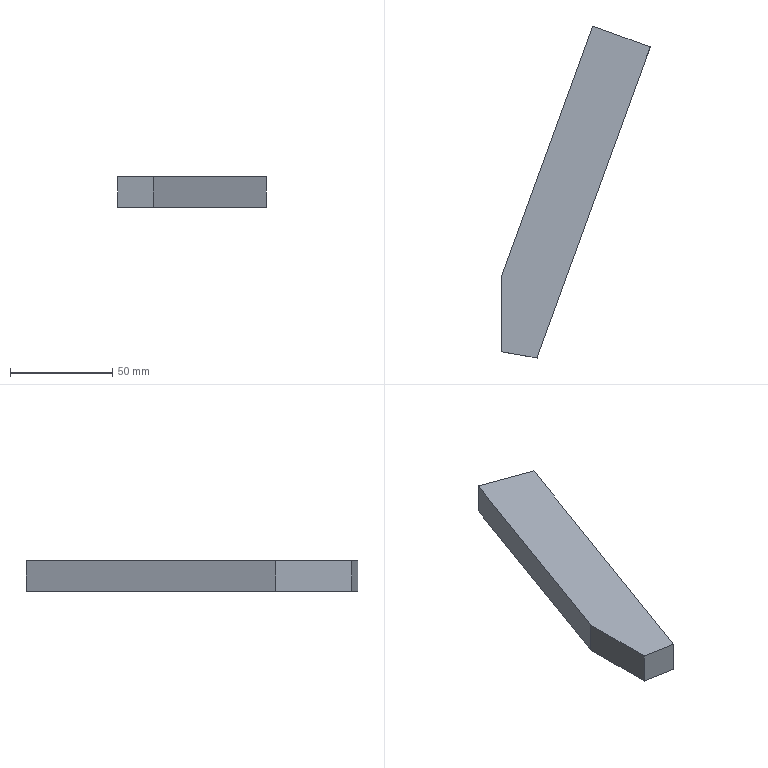Part | NX | features solid 2 | 1 solid | 7 faces | box 72.653 x 162.455 x 15 mm | volume 70513 mm3 | plane 7
STEP:
#1=CARTESIAN_POINT('',(650.,25.,0.));
#2=VERTEX_POINT('',#1);
#3=CARTESIAN_POINT('',(650.,25.,15.));
#4=VERTEX_POINT('',#3);
#5=CARTESIAN_POINT('',(650.,25.,0.));
#6=DIRECTION('',(0.,0.,1.));
#7=VECTOR('',#6,1000.);
#8=LINE('',#5,#7);
#9=EDGE_CURVE('',#2,#4,#8,.T.);
#10=ORIENTED_EDGE('',*,*,#9,.T.);
#11=CARTESIAN_POINT('',(694.463,147.16,15.));
#12=VERTEX_POINT('',#11);
#13=CARTESIAN_POINT('',(660.261,53.191,15.));
#14=DIRECTION('',(0.342,0.9397,0.));
#15=VECTOR('',#14,1000.);
#16=LINE('',#13,#15);
#17=EDGE_CURVE('',#12,#4,#16,.F.);
#18=ORIENTED_EDGE('',*,*,#17,.F.);
#19=CARTESIAN_POINT('',(694.463,147.16,0.));
#20=VERTEX_POINT('',#19);
#21=CARTESIAN_POINT('',(694.463,147.16,0.));
#22=DIRECTION('',(0.,0.,-1.));
#23=VECTOR('',#22,1000.);
#24=LINE('',#21,#23);
#25=EDGE_CURVE('',#20,#12,#24,.F.);
#26=ORIENTED_EDGE('',*,*,#25,.F.);
#27=CARTESIAN_POINT('',(660.261,53.191,0.));
#28=DIRECTION('',(-0.342,-0.9397,0.));
#29=VECTOR('',#28,1000.);
#30=LINE('',#27,#29);
#31=EDGE_CURVE('',#20,#2,#30,.T.);
#32=ORIENTED_EDGE('',*,*,#31,.T.);
#33=EDGE_LOOP('',(#10,#18,#26,#32));
#34=FACE_BOUND('',#33,.T.);
#35=CARTESIAN_POINT('',(660.261,53.191,0.));
#36=DIRECTION('',(-0.9397,0.342,0.));
#37=DIRECTION('',(-0.342,-0.9397,0.));
#38=AXIS2_PLACEMENT_3D('',#35,#36,#37);
#39=PLANE('',#38);
#40=ADVANCED_FACE('',(#34),#39,.T.);
#41=ORIENTED_EDGE('',*,*,#25,.T.);
#42=CARTESIAN_POINT('',(722.653,136.899,15.));
#43=VERTEX_POINT('',#42);
#44=CARTESIAN_POINT('',(694.463,147.16,15.));
#45=DIRECTION('',(0.9397,-0.342,0.));
#46=VECTOR('',#45,1000.);
#47=LINE('',#44,#46);
#48=EDGE_CURVE('',#12,#43,#47,.T.);
#49=ORIENTED_EDGE('',*,*,#48,.T.);
#50=CARTESIAN_POINT('',(722.653,136.899,0.));
#51=VERTEX_POINT('',#50);
#52=CARTESIAN_POINT('',(722.653,136.899,0.));
#53=DIRECTION('',(0.,0.,1.));
#54=VECTOR('',#53,1000.);
#55=LINE('',#52,#54);
#56=EDGE_CURVE('',#51,#43,#55,.T.);
#57=ORIENTED_EDGE('',*,*,#56,.F.);
#58=CARTESIAN_POINT('',(694.463,147.16,0.));
#59=DIRECTION('',(0.9397,-0.342,0.));
#60=VECTOR('',#59,1000.);
#61=LINE('',#58,#60);
#62=EDGE_CURVE('',#20,#51,#61,.T.);
#63=ORIENTED_EDGE('',*,*,#62,.F.);
#64=EDGE_LOOP('',(#41,#49,#57,#63));
#65=FACE_BOUND('',#64,.T.);
#66=CARTESIAN_POINT('',(694.463,147.16,0.));
#67=DIRECTION('',(-0.342,-0.9397,0.));
#68=DIRECTION('',(0.9397,-0.342,0.));
#69=AXIS2_PLACEMENT_3D('',#66,#67,#68);
#70=PLANE('',#69);
#71=ADVANCED_FACE('',(#65),#70,.F.);
#72=CARTESIAN_POINT('',(667.259,-15.295,15.));
#73=VERTEX_POINT('',#72);
#74=CARTESIAN_POINT('',(688.451,42.93,15.));
#75=DIRECTION('',(0.342,0.9397,0.));
#76=VECTOR('',#75,1000.);
#77=LINE('',#74,#76);
#78=EDGE_CURVE('',#43,#73,#77,.F.);
#79=ORIENTED_EDGE('',*,*,#78,.T.);
#80=CARTESIAN_POINT('',(667.259,-15.295,0.));
#81=VERTEX_POINT('',#80);
#82=CARTESIAN_POINT('',(667.259,-15.295,-25.));
#83=DIRECTION('',(0.,0.,-1.));
#84=VECTOR('',#83,1000.);
#85=LINE('',#82,#84);
#86=EDGE_CURVE('',#73,#81,#85,.T.);
#87=ORIENTED_EDGE('',*,*,#86,.T.);
#88=CARTESIAN_POINT('',(688.451,42.93,0.));
#89=DIRECTION('',(-0.342,-0.9397,0.));
#90=VECTOR('',#89,1000.);
#91=LINE('',#88,#90);
#92=EDGE_CURVE('',#51,#81,#91,.T.);
#93=ORIENTED_EDGE('',*,*,#92,.F.);
#94=ORIENTED_EDGE('',*,*,#56,.T.);
#95=EDGE_LOOP('',(#79,#87,#93,#94));
#96=FACE_BOUND('',#95,.T.);
#97=CARTESIAN_POINT('',(688.451,42.93,0.));
#98=DIRECTION('',(-0.9397,0.342,0.));
#99=DIRECTION('',(-0.342,-0.9397,0.));
#100=AXIS2_PLACEMENT_3D('',#97,#98,#99);
#101=PLANE('',#100);
#102=ADVANCED_FACE('',(#96),#101,.F.);
#103=CARTESIAN_POINT('',(650.,-12.251,0.));
#104=VERTEX_POINT('',#103);
#105=CARTESIAN_POINT('',(650.,-30.,0.));
#106=DIRECTION('',(0.,1.,0.));
#107=VECTOR('',#106,1000.);
#108=LINE('',#105,#107);
#109=EDGE_CURVE('',#2,#104,#108,.F.);
#110=ORIENTED_EDGE('',*,*,#109,.T.);
#111=CARTESIAN_POINT('',(650.,-12.251,15.));
#112=VERTEX_POINT('',#111);
#113=CARTESIAN_POINT('',(650.,-12.251,-25.));
#114=DIRECTION('',(0.,0.,-1.));
#115=VECTOR('',#114,1000.);
#116=LINE('',#113,#115);
#117=EDGE_CURVE('',#104,#112,#116,.F.);
#118=ORIENTED_EDGE('',*,*,#117,.T.);
#119=CARTESIAN_POINT('',(650.,-30.,15.));
#120=DIRECTION('',(0.,1.,0.));
#121=VECTOR('',#120,1000.);
#122=LINE('',#119,#121);
#123=EDGE_CURVE('',#4,#112,#122,.F.);
#124=ORIENTED_EDGE('',*,*,#123,.F.);
#125=ORIENTED_EDGE('',*,*,#9,.F.);
#126=EDGE_LOOP('',(#110,#118,#124,#125));
#127=FACE_BOUND('',#126,.T.);
#128=CARTESIAN_POINT('',(650.,-30.,-25.));
#129=DIRECTION('',(-1.,0.,0.));
#130=DIRECTION('',(0.,-1.,0.));
#131=AXIS2_PLACEMENT_3D('',#128,#129,#130);
#132=PLANE('',#131);
#133=ADVANCED_FACE('',(#127),#132,.T.);
#134=ORIENTED_EDGE('',*,*,#123,.T.);
#135=CARTESIAN_POINT('',(648.76,-12.033,15.));
#136=DIRECTION('',(0.9848,-0.1736,0.));
#137=VECTOR('',#136,1000.);
#138=LINE('',#135,#137);
#139=EDGE_CURVE('',#112,#73,#138,.T.);
#140=ORIENTED_EDGE('',*,*,#139,.T.);
#141=ORIENTED_EDGE('',*,*,#78,.F.);
#142=ORIENTED_EDGE('',*,*,#48,.F.);
#143=ORIENTED_EDGE('',*,*,#17,.T.);
#144=EDGE_LOOP('',(#134,#140,#141,#142,#143));
#145=FACE_BOUND('',#144,.T.);
#146=CARTESIAN_POINT('',(660.261,53.191,15.));
#147=DIRECTION('',(0.,0.,1.));
#148=DIRECTION('',(0.342,0.9397,0.));
#149=AXIS2_PLACEMENT_3D('',#146,#147,#148);
#150=PLANE('',#149);
#151=ADVANCED_FACE('',(#145),#150,.T.);
#152=ORIENTED_EDGE('',*,*,#92,.T.);
#153=CARTESIAN_POINT('',(655.209,-13.17,0.));
#154=DIRECTION('',(-0.9848,0.1736,0.));
#155=VECTOR('',#154,1000.);
#156=LINE('',#153,#155);
#157=EDGE_CURVE('',#81,#104,#156,.T.);
#158=ORIENTED_EDGE('',*,*,#157,.T.);
#159=ORIENTED_EDGE('',*,*,#109,.F.);
#160=ORIENTED_EDGE('',*,*,#31,.F.);
#161=ORIENTED_EDGE('',*,*,#62,.T.);
#162=EDGE_LOOP('',(#152,#158,#159,#160,#161));
#163=FACE_BOUND('',#162,.T.);
#164=CARTESIAN_POINT('',(660.261,53.191,0.));
#165=DIRECTION('',(0.,0.,1.));
#166=DIRECTION('',(0.342,0.9397,0.));
#167=AXIS2_PLACEMENT_3D('',#164,#165,#166);
#168=PLANE('',#167);
#169=ADVANCED_FACE('',(#163),#168,.F.);
#170=ORIENTED_EDGE('',*,*,#157,.F.);
#171=ORIENTED_EDGE('',*,*,#86,.F.);
#172=ORIENTED_EDGE('',*,*,#139,.F.);
#173=ORIENTED_EDGE('',*,*,#117,.F.);
#174=EDGE_LOOP('',(#170,#171,#172,#173));
#175=FACE_BOUND('',#174,.T.);
#176=CARTESIAN_POINT('',(655.209,-13.17,-25.));
#177=DIRECTION('',(-0.1736,-0.9848,0.));
#178=DIRECTION('',(0.9848,-0.1736,0.));
#179=AXIS2_PLACEMENT_3D('',#176,#177,#178);
#180=PLANE('',#179);
#181=ADVANCED_FACE('',(#175),#180,.T.);
#182=CLOSED_SHELL('',(#40,#71,#102,#133,#151,#169,#181));
#183=MANIFOLD_SOLID_BREP('',#182);
#184=(LENGTH_UNIT()NAMED_UNIT(*)SI_UNIT(.MILLI.,.METRE.));
#185=UNCERTAINTY_MEASURE_WITH_UNIT(LENGTH_MEASURE(0.00001),#184,'','');
#186=(NAMED_UNIT(*)PLANE_ANGLE_UNIT()SI_UNIT($,.RADIAN.));
#187=(NAMED_UNIT(*)SI_UNIT($,.STERADIAN.)SOLID_ANGLE_UNIT());
#188=(GEOMETRIC_REPRESENTATION_CONTEXT(3)GLOBAL_UNCERTAINTY_ASSIGNED_CONTEXT((#185))GLOBAL_UNIT_ASSIGNED_CONTEXT((#184,#186,#187))REPRESENTATION_CONTEXT('',''));
#189=ADVANCED_BREP_SHAPE_REPRESENTATION('',(#183),#188);